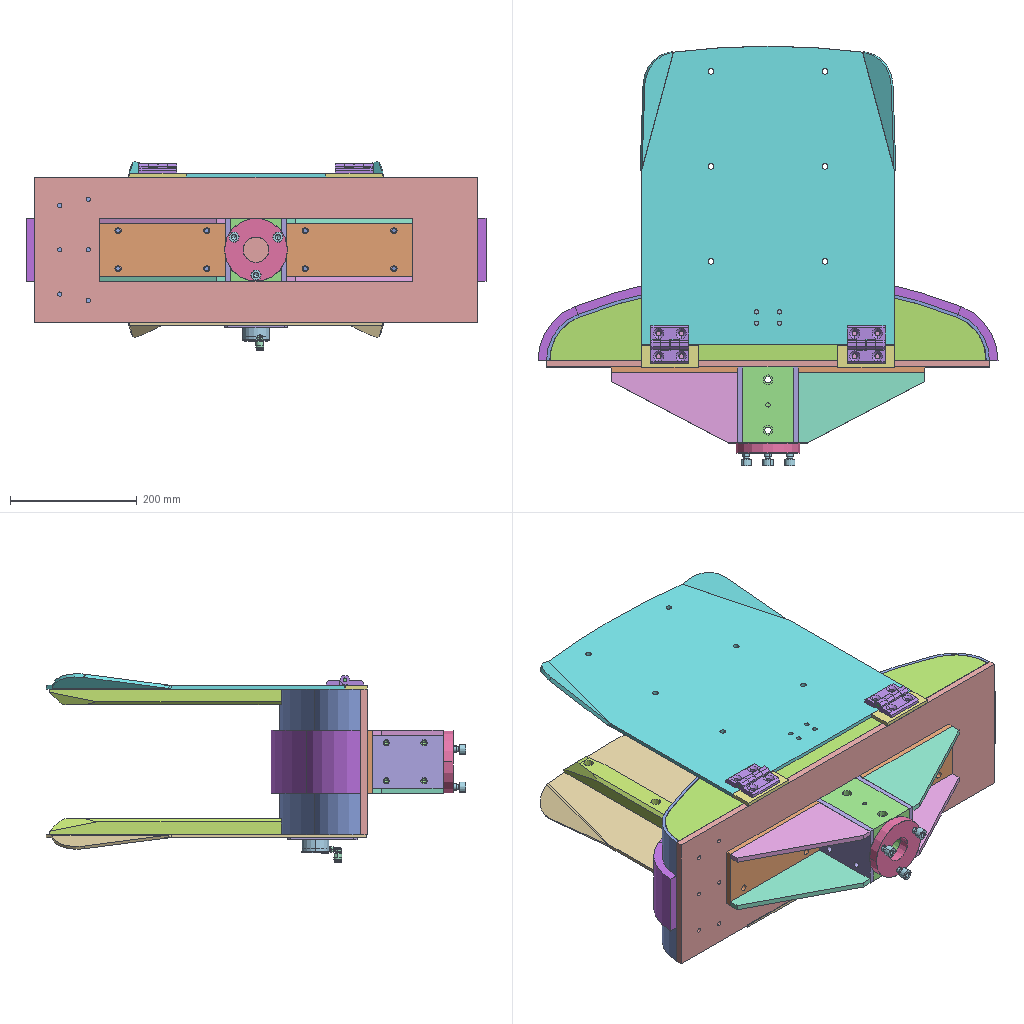Assembly | SolidWorks | 29 different items | 44 placed | box 727 x 663 x 298 mm
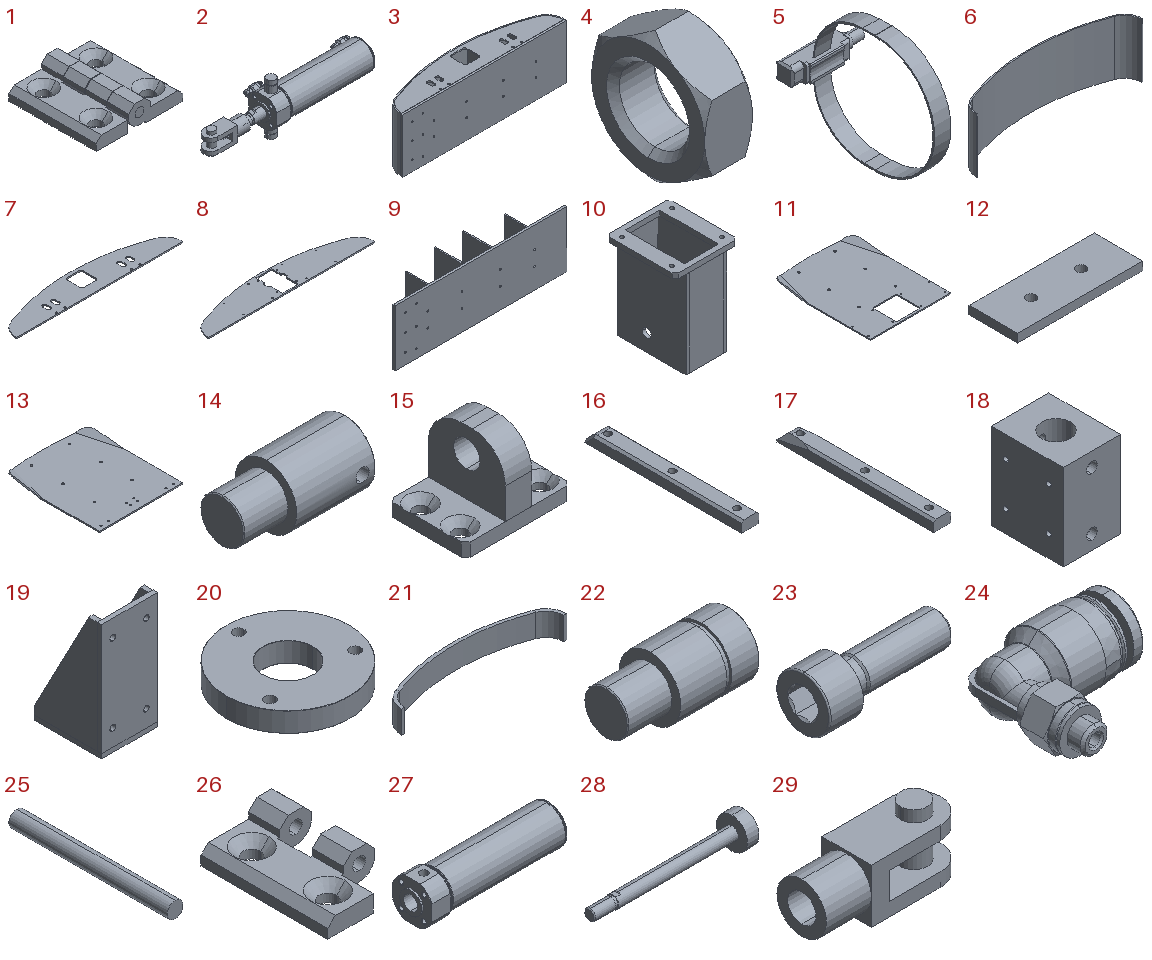Parts list (item | name | quantity | parent item | size | volume | features):
1 | (subassembly) | x2 | - | 60 x 60 x 15 mm | 28445 mm3 | -
2 | (subassembly) | x1 | - | 261.082 x 64.35 x 80 mm | 157022 mm3 | features ReferencePattern 2, LocalLPattern 1
3 | (subassembly) | x1 | - | 700.002 x 139 x 230 mm | 3599547 mm3 | features AEMSimFeature 1
4 | - | x1 | in 2 | 8 x 19 x 21.939 mm | 1553 mm3 | features BaseBody 1
5 | - | x1 | in 2 | 30 x 54.5 x 46 mm | 1772 mm3 | features BaseBody 1
6 | - | x1 | in 3 | 700.002 x 128.973 x 230 mm | 913627 mm3 | features FlatPattern 1, ICE 1, SMBaseFlange 1, SheetMetal 1
7 | - | x1 | in 3 | 688.178 x 124 x 5 mm | 305727 mm3 | features ICE 3, Fillet 1, FlatPattern 1, SMBaseFlange 1, SheetMetal 1
8 | - | x1 | in 3 | 688.178 x 124 x 5 mm | 300076 mm3 | features HoleWzd 2, ICE 2, Fillet 1, FlatPattern 1, SMBaseFlange 1, SheetMetal 1
9 | - | x1 | in 3 | 700 x 131 x 230 mm | 2080116 mm3 | features HoleWzd 3, ICE 2, Extrusion 1
10 | - | x1 | - | 100 x 110 x 148 mm | 274855 mm3 | features ICE 4, Chamfer 1, Extrusion 1, HoleWzd 1
11 | - | x1 | - | 403.29 x 506.284 x 23.281 mm | 923449 mm3 | features ICE 5, HoleWzd 2, Chamfer 1, EdgeFlange 1, Fillet 1, FlatPattern 1, SM3dBend 1, SMBaseFlange 1, SheetMetal 1
12 | - | x2 | - | 90 x 35 x 6 mm | 18438 mm3 | features Extrusion 1, HoleWzd 1
13 | - | x1 | - | 403.952 x 471.784 x 24.242 mm | 1111640 mm3 | features HoleWzd 3, Fillet 2, ICE 2, SM3dBend 2, FlatPattern 1, SMBaseFlange 1, SheetMetal 1
14 | - | x2 | in 2 | 28 x 14 x 14 mm | 3456 mm3 | features Chamfer 2, ICE 2, Revolution 1
15 | - | x1 | - | 48 x 35 x 35 mm | 18352 mm3 | features ICE 2, Chamfer 1, Extrusion 1, Fillet 1, HoleWzd 1
16 | - | x1 | - | 40 x 366 x 25 mm | 339646 mm3 | features Chamfer 4, Fillet 4, ICE 3, HoleWzd 2, Extrusion 1
17 | - | x4 | - | 40 x 366 x 25 mm | 336902 mm3 | features Chamfer 5, ICE 5, Fillet 3, HoleWzd 2, Extrusion 1, MirrorPattern 1
18 | - | x1 | - | 80 x 100 x 120 mm | 786189 mm3 | features HoleWzd 5, ICE 4, Extrusion 1
19 | - | x2 | - | 100 x 120 x 208 mm | 465813 mm3 | features ICE 5, HoleWzd 3, Extrusion 1
20 | - | x1 | - | 100 x 100 x 16 mm | 102816 mm3 | features Chamfer 1, CirPattern 1, Extrusion 1, HoleWzd 1
21 | - | x1 | - | 727 x 142.5 x 100 mm | 1111821 mm3 | features FlatPattern 1, HoleWzd 1, ICE 1, SMBaseFlange 1, SheetMetal 1
22 | - | x2 | in 2 | 28 x 14 x 14 mm | 3531 mm3 | features Chamfer 2, ICE 2, RevCut 1, Revolution 1
23 | - | x3 | - | 40 x 16 x 16 mm | 3907 mm3 | features RevCut 2, Revolution 2, Chamfer 1, Cut 1, Fillet 1
24 | - | x2 | in 2 | 24.619 x 23.25 x 12.5 mm | 2103 mm3 | features BaseBody 1
25 | - | x2 | in 1 | 6 x 60 x 6 mm | 1696 mm3 | features BaseBody 1
26 | - | x4 | in 1 | 37.5 x 60 x 15 mm | 13374 mm3 | features BaseBody 1
27 | - | x1 | in 2 | 157 x 44 x 44 mm | 70964 mm3 | features HoleWzd 2, BaseBody 1, ICE 1
28 | - | x1 | in 2 | 198 x 40 x 40 mm | 54072 mm3 | features BaseBody 1
29 | - | x1 | in 2 | 62 x 22 x 34 mm | 19162 mm3 | features ICE 4, Extrusion 1, Fillet 1, HoleWzd 1
Mates (type | each side: item.copy, entity, surface, feature):
In the top assembly
Coincident | 8.1 face plane Base-Flange1 | 10.1 face plane Boss-Extrude1
Concentric | 10.1 face cylinder Cut-Extrude2 | 14.1 face cylinder Revolve1
Width | 10.1 face plane Boss-Extrude2 | 10.1 face plane Boss-Extrude2 | 27.1 face cylinder Input1
Coincident | 7.1 face plane Base-Flange1 | 13.1 face plane Base-Flange1
DistanceDim | 13.1 face plane Base-Flange1 | 7.1 face plane Base-Flange1
Coincident | 13.1 face plane Base-Flange1 | 26.1 face plane Input1
DistanceDim | 7.1 face plane Base-Flange1 | 26.2 face plane Input1
Width | 13.1 face plane Base-Flange1 | 13.1 face plane Base-Flange1 | 9.1 face plane Boss-Extrude1 | 9.1 face plane Boss-Extrude1
Coincident | 26.1 face plane Input1 | 26.3 face plane Input1 | 2 times
DistanceDim | 26.3 face plane Input1 | 13.1 face plane Base-Flange1
Coincident | 13.1 face plane Base-Flange1 | 15.1 face plane Boss-Extrude1
Concentric | 13.1 face cylinder M6 Clearance Hole2 | 15.1 face cylinder Hole Size slotted raised countersunk screw type 1 | 2 times
Coincident | 13.1 face plane Base-Flange1 | 17.1 face plane Boss-Extrude1
Concentric | 13.1 face cylinder M8 Clearance Hole1 | 17.1 face cylinder Hole Size (based on) hex socket cap screw type 1 | 2 times
Coincident | 9.1 face plane Boss-Extrude1 | 19.1 face plane Boss-Extrude4
Concentric | 9.1 face cylinder M8 Tapped Hole1 | 19.1 face cylinder M8 Clearance Hole1 | 2 times
Coincident | 9.1 face plane Boss-Extrude1 | 19.2 face plane Boss-Extrude4
Concentric | 9.1 face cylinder M8 Tapped Hole1 | 19.2 face cylinder M8 Clearance Hole1 | 2 times
Coincident | 19.2 face plane Boss-Extrude1 | 18.1 face plane Boss-Extrude1
Concentric | 19.2 face cylinder M8 Clearance Hole2 | 18.1 face cylinder M8 Tapped Hole2 | 2 times
Coincident | 18.1 face plane Boss-Extrude1 | 20.1 face plane Boss-Extrude1
Concentric | 18.1 face cylinder Cut-Extrude1 | 20.1 face cylinder Boss-Extrude1
Coincident | 8.1 face plane Base-Flange1 | 11.1 face plane Base-Flange1
Concentric | 8.1 face cylinder M5 Tapped Hole2 | 11.1 face cylinder M5 Clearance Hole1 | 2 times
Coincident | 11.1 face plane Base-Flange1 | 17.2 face plane Boss-Extrude1
Concentric | 11.1 face cylinder M8 Clearance Hole1 | 17.2 face cylinder Hole Size (based on) hex socket cap screw type 1 | 2 times
Concentric | 20.1 face cylinder CirPattern1 | 23.1 face cylinder Base-Revolve
DistanceDim | 23.1 face plane Base-Revolve | 20.1 face plane Boss-Extrude1
Concentric | 8.1 face cylinder M5 Tapped Hole1 | 10.1 face cylinder M5 Clearance Hole1 | 2 times
Concentric | 15.2 face | assembly face
Coincident | 15.2 face | assembly face
Parallel | 13.1 face cylinder M6 Clearance Hole1 | 26.1 face cylinder Input1
DistanceDim | 26.1 face plane Input1 | 13.1 face plane Base-Flange1
Coincident | 7.1 face plane Base-Flange1 | 12.1 face plane Boss-Extrude1
Concentric | 7.1 face cylinder Cut-Extrude3 | 12.1 face cylinder M6 Clearance Hole1 | 2 times
Coincident | 7.1 face plane Base-Flange1 | 12.2 face plane Boss-Extrude1
Concentric | 7.1 face cylinder Cut-Extrude3 | 12.2 face cylinder M6 Clearance Hole1 | 2 times
Coincident | 11.1 face plane Base-Flange1 | 16.1 face
Concentric | 11.1 face cylinder M8 Clearance Hole1 | 16.1 face | 2 times
Coincident | 13.1 face plane Base-Flange1 | 16.2 face
Concentric | 13.1 face cylinder M8 Clearance Hole1 | 16.2 face | 2 times
Coincident | 13.1 face plane Base-Flange1 | 17.3 face plane Boss-Extrude1
Concentric | 13.1 face cylinder M8 Clearance Hole1 | 17.3 face cylinder Cut-Extrude1 | 2 times
Coincident | 11.1 face plane Base-Flange1 | 17.4 face plane Boss-Extrude1
Concentric | 11.1 face cylinder M8 Clearance Hole1 | 17.4 face cylinder Cut-Extrude1
Concentric | 11.1 edge | 17.4 face cylinder Cut-Extrude1
Concentric | 6.1 face cylinder Base Bend4 | 21.1 face cylinder Base Bend4
Width | 21.1 face plane Base Bend4 | 21.1 face plane Base Bend4 | 7.1 face plane Base-Flange1 | 8.1 face plane Base-Flange1
In subassembly 2
Coincident | 27.2 face plane Input1 | 24.1 face plane Input1
Concentric | 27.2 face cylinder Input1 | 24.1 face cylinder Input1
Coincident | 27.2 face plane Input1 | 14.2 face plane Revolve1
Concentric | 27.2 face cylinder M10x1.25 Tapped Hole1 | 14.2 face cylinder Revolve1
Coincident | 27.2 face plane Input1 | 14.3 face plane Revolve1
Concentric | 27.2 face cylinder M10x1.25 Tapped Hole2 | 14.3 face cylinder Revolve1
DistanceDim | 29.1 face plane Boss-Extrude1 | 28.1 face plane Input1
Concentric | 28.1 face cylinder Input1 | 29.1 face cylinder Cut-Extrude6
Parallel | 27.2 face plane Input1 | 29.1 face plane Boss-Extrude1
Concentric | 27.2 face cylinder Input1 | 5.1 face
Coincident | 27.2 face plane Input1 | 5.1 face
Concentric | 27.2 face cylinder Input1 | 5.2 face
Coincident | 27.2 face plane Input1 | 22.1 face plane Revolve1
Concentric | 27.2 face cylinder M10x1.25 Tapped Hole2 | 22.1 face cylinder Revolve1
Coincident | 27.2 face plane Input1 | 22.2 face plane Revolve1
Concentric | 27.2 face cylinder M10x1.25 Tapped Hole1 | 22.2 face cylinder Revolve1
In subassembly 3
Coincident | 9.2 face plane Boss-Extrude1 | 8.2 face plane Base-Flange1 | 2 times
Coincident | 9.2 face plane Boss-Extrude1 | 7.2 face plane Base-Flange1 | 2 times
Coincident | 7.2 face plane Cut-Extrude1 | 8.2 face plane Cut-Extrude1
Coincident | 6.2 face plane Base Bend4 | 8.2 face plane Base-Flange1
Concentric | 6.2 face cylinder Base Bend4 | 8.2 face cylinder Base-Flange1
DistanceDim | 7.2 edge | 9.2 face plane Boss-Extrude1
Coincident | 9.2 face plane Boss-Extrude1 | 6.2 edge